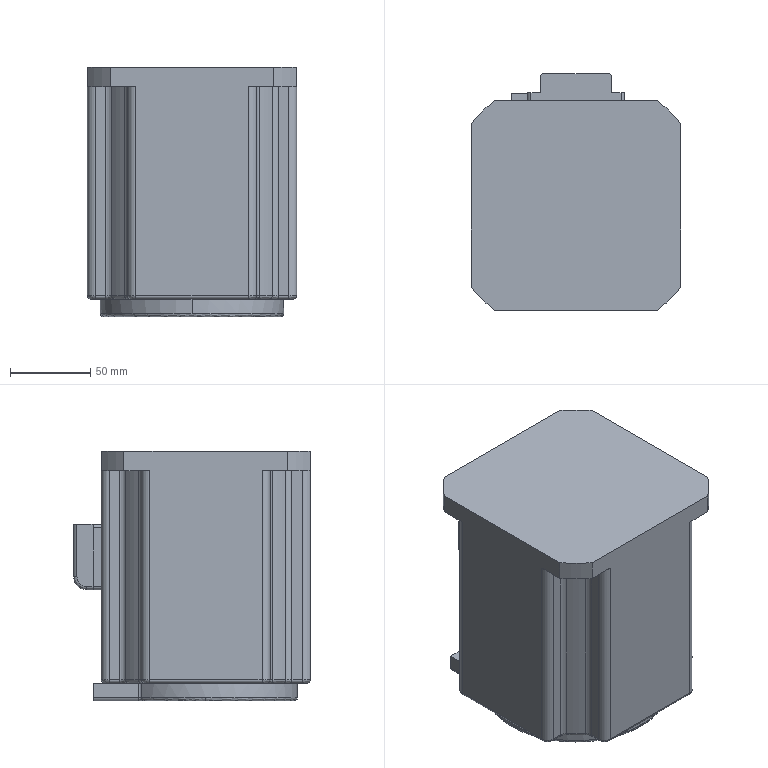Part | STEP file | Link3_J3mot | 1 solid | 112 faces | box 130 x 147 x 155 mm | volume 2279615 mm3 | cylinder 53 | plane 32 | spline 27 | commonest cylinder face diameters 4 x25 10 x16 130 x4 165 x4 114 x3 16 x1